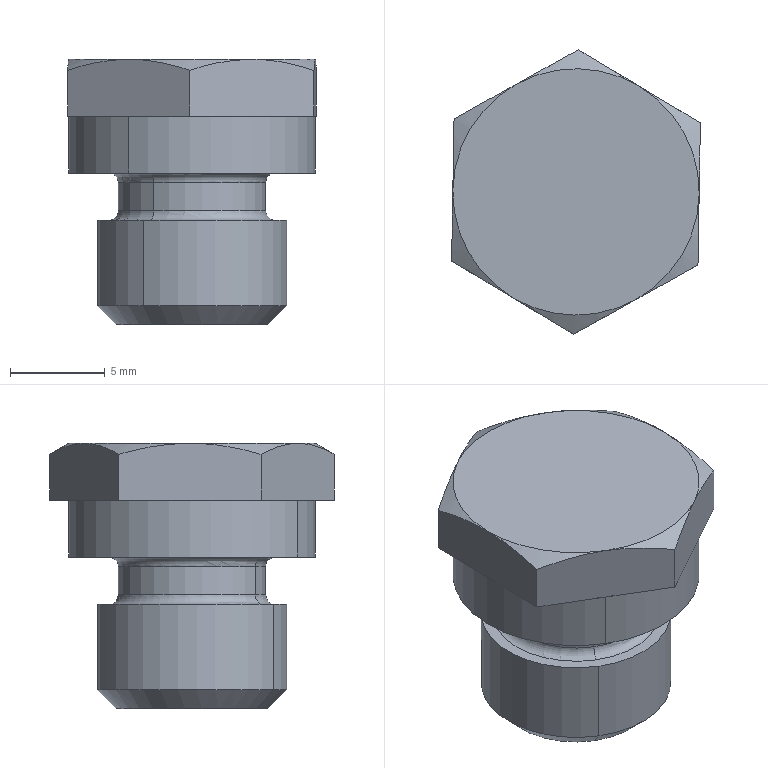Part | SolidWorks | features BaseBody 1 | 1 solid | 34 faces | box 13.126 x 15.009 x 14 mm | volume 1374 mm3 | plane 16 | cone 8 | cylinder 6 | torus 4 | commonest cylinder face diameters 7.8 x2 10 x2 13 x2
STEP:
#1=CARTESIAN_POINT('',(388.093,181.656,45.));
#2=VERTEX_POINT('',#1);
#3=CARTESIAN_POINT('',(392.107,188.344,45.));
#4=VERTEX_POINT('',#3);
#5=CARTESIAN_POINT('',(390.1,185.,45.));
#6=DIRECTION('',(0.,0.,-1.));
#7=DIRECTION('',(0.5146,0.8574,0.));
#8=AXIS2_PLACEMENT_3D('',#5,#6,#7);
#9=CIRCLE('',#8,3.9);
#10=EDGE_CURVE('',#2,#4,#9,.T.);
#11=ORIENTED_EDGE('',*,*,#10,.F.);
#12=CARTESIAN_POINT('',(387.836,181.227,45.5));
#13=VERTEX_POINT('',#12);
#14=CARTESIAN_POINT('',(387.836,181.227,45.));
#15=DIRECTION('',(0.8574,-0.5146,0.));
#16=DIRECTION('',(0.5146,0.8574,0.));
#17=AXIS2_PLACEMENT_3D('',#14,#15,#16);
#18=CIRCLE('',#17,0.5);
#19=EDGE_CURVE('',#2,#13,#18,.T.);
#20=ORIENTED_EDGE('',*,*,#19,.T.);
#21=CARTESIAN_POINT('',(392.364,188.773,45.5));
#22=VERTEX_POINT('',#21);
#23=CARTESIAN_POINT('',(390.1,185.,45.5));
#24=DIRECTION('',(0.,0.,1.));
#25=DIRECTION('',(0.5146,0.8574,0.));
#26=AXIS2_PLACEMENT_3D('',#23,#24,#25);
#27=CIRCLE('',#26,4.4);
#28=EDGE_CURVE('',#22,#13,#27,.T.);
#29=ORIENTED_EDGE('',*,*,#28,.F.);
#30=CARTESIAN_POINT('',(392.364,188.773,45.));
#31=DIRECTION('',(-0.8574,0.5146,0.));
#32=DIRECTION('',(-0.5146,-0.8574,0.));
#33=AXIS2_PLACEMENT_3D('',#30,#31,#32);
#34=CIRCLE('',#33,0.5);
#35=EDGE_CURVE('',#4,#22,#34,.T.);
#36=ORIENTED_EDGE('',*,*,#35,.F.);
#37=EDGE_LOOP('',(#11,#20,#29,#36));
#38=FACE_OUTER_BOUND('',#37,.T.);
#39=CARTESIAN_POINT('',(390.1,185.,45.));
#40=DIRECTION('',(0.,0.,-1.));
#41=DIRECTION('',(0.5146,0.8574,0.));
#42=AXIS2_PLACEMENT_3D('',#39,#40,#41);
#43=TOROIDAL_SURFACE('',#42,4.4,0.5);
#44=ADVANCED_FACE('',(#38),#43,.F.);
#45=CARTESIAN_POINT('',(392.107,188.344,43.5));
#46=VERTEX_POINT('',#45);
#47=CARTESIAN_POINT('',(388.093,181.656,43.5));
#48=VERTEX_POINT('',#47);
#49=CARTESIAN_POINT('',(390.1,185.,43.5));
#50=DIRECTION('',(0.,0.,1.));
#51=DIRECTION('',(-0.5146,-0.8574,0.));
#52=AXIS2_PLACEMENT_3D('',#49,#50,#51);
#53=CIRCLE('',#52,3.9);
#54=EDGE_CURVE('',#46,#48,#53,.T.);
#55=ORIENTED_EDGE('',*,*,#54,.F.);
#56=CARTESIAN_POINT('',(392.364,188.773,43.));
#57=VERTEX_POINT('',#56);
#58=CARTESIAN_POINT('',(392.364,188.773,43.5));
#59=DIRECTION('',(0.8574,-0.5146,0.));
#60=DIRECTION('',(0.5146,0.8574,0.));
#61=AXIS2_PLACEMENT_3D('',#58,#59,#60);
#62=CIRCLE('',#61,0.5);
#63=EDGE_CURVE('',#46,#57,#62,.T.);
#64=ORIENTED_EDGE('',*,*,#63,.T.);
#65=CARTESIAN_POINT('',(387.836,181.227,43.));
#66=VERTEX_POINT('',#65);
#67=CARTESIAN_POINT('',(390.1,185.,43.));
#68=DIRECTION('',(0.,0.,-1.));
#69=DIRECTION('',(-0.5146,-0.8574,0.));
#70=AXIS2_PLACEMENT_3D('',#67,#68,#69);
#71=CIRCLE('',#70,4.4);
#72=EDGE_CURVE('',#66,#57,#71,.T.);
#73=ORIENTED_EDGE('',*,*,#72,.F.);
#74=CARTESIAN_POINT('',(387.836,181.227,43.5));
#75=DIRECTION('',(-0.8574,0.5146,0.));
#76=DIRECTION('',(-0.5146,-0.8574,0.));
#77=AXIS2_PLACEMENT_3D('',#74,#75,#76);
#78=CIRCLE('',#77,0.5);
#79=EDGE_CURVE('',#48,#66,#78,.T.);
#80=ORIENTED_EDGE('',*,*,#79,.F.);
#81=EDGE_LOOP('',(#55,#64,#73,#80));
#82=FACE_OUTER_BOUND('',#81,.T.);
#83=CARTESIAN_POINT('',(390.1,185.,43.5));
#84=DIRECTION('',(0.,0.,1.));
#85=DIRECTION('',(-0.5146,-0.8574,0.));
#86=AXIS2_PLACEMENT_3D('',#83,#84,#85);
#87=TOROIDAL_SURFACE('',#86,4.4,0.5);
#88=ADVANCED_FACE('',(#82),#87,.F.);
#89=CARTESIAN_POINT('',(392.159,188.43,37.5));
#90=VERTEX_POINT('',#89);
#91=CARTESIAN_POINT('',(388.041,181.57,37.5));
#92=VERTEX_POINT('',#91);
#93=CARTESIAN_POINT('',(390.1,185.,37.5));
#94=DIRECTION('',(0.,0.,-1.));
#95=DIRECTION('',(0.5146,0.8574,0.));
#96=AXIS2_PLACEMENT_3D('',#93,#94,#95);
#97=CIRCLE('',#96,4.);
#98=EDGE_CURVE('',#90,#92,#97,.T.);
#99=ORIENTED_EDGE('',*,*,#98,.F.);
#100=CARTESIAN_POINT('',(392.673,189.287,38.5));
#101=VERTEX_POINT('',#100);
#102=CARTESIAN_POINT('',(392.159,188.43,37.5));
#103=DIRECTION('',(0.3639,0.6063,0.7071));
#104=VECTOR('',#103,1000.);
#105=LINE('',#102,#104);
#106=EDGE_CURVE('',#90,#101,#105,.T.);
#107=ORIENTED_EDGE('',*,*,#106,.T.);
#108=CARTESIAN_POINT('',(387.527,180.713,38.5));
#109=VERTEX_POINT('',#108);
#110=CARTESIAN_POINT('',(390.1,185.,38.5));
#111=DIRECTION('',(0.,0.,1.));
#112=DIRECTION('',(0.5146,0.8574,0.));
#113=AXIS2_PLACEMENT_3D('',#110,#111,#112);
#114=CIRCLE('',#113,5.);
#115=EDGE_CURVE('',#109,#101,#114,.T.);
#116=ORIENTED_EDGE('',*,*,#115,.F.);
#117=CARTESIAN_POINT('',(388.041,181.57,37.5));
#118=DIRECTION('',(-0.3639,-0.6063,0.7071));
#119=VECTOR('',#118,1000.);
#120=LINE('',#117,#119);
#121=EDGE_CURVE('',#92,#109,#120,.T.);
#122=ORIENTED_EDGE('',*,*,#121,.F.);
#123=EDGE_LOOP('',(#99,#107,#116,#122));
#124=FACE_OUTER_BOUND('',#123,.T.);
#125=CARTESIAN_POINT('',(390.1,185.,37.5));
#126=DIRECTION('',(0.,0.,1.));
#127=DIRECTION('',(-0.5146,-0.8574,0.));
#128=AXIS2_PLACEMENT_3D('',#125,#126,#127);
#129=CONICAL_SURFACE('',#128,4.,0.7854);
#130=ADVANCED_FACE('',(#124),#129,.T.);
#131=CARTESIAN_POINT('',(392.673,189.287,43.));
#132=VERTEX_POINT('',#131);
#133=CARTESIAN_POINT('',(387.527,180.713,43.));
#134=VERTEX_POINT('',#133);
#135=CARTESIAN_POINT('',(390.1,185.,43.));
#136=DIRECTION('',(0.,0.,-1.));
#137=DIRECTION('',(0.5146,0.8574,0.));
#138=AXIS2_PLACEMENT_3D('',#135,#136,#137);
#139=CIRCLE('',#138,5.);
#140=EDGE_CURVE('',#132,#134,#139,.T.);
#141=ORIENTED_EDGE('',*,*,#140,.T.);
#142=CARTESIAN_POINT('',(387.527,180.713,45.5));
#143=DIRECTION('',(0.,0.,-1.));
#144=VECTOR('',#143,1000.);
#145=LINE('',#142,#144);
#146=EDGE_CURVE('',#134,#109,#145,.T.);
#147=ORIENTED_EDGE('',*,*,#146,.T.);
#148=ORIENTED_EDGE('',*,*,#115,.T.);
#149=CARTESIAN_POINT('',(392.673,189.287,45.5));
#150=DIRECTION('',(0.,0.,-1.));
#151=VECTOR('',#150,1000.);
#152=LINE('',#149,#151);
#153=EDGE_CURVE('',#132,#101,#152,.T.);
#154=ORIENTED_EDGE('',*,*,#153,.F.);
#155=EDGE_LOOP('',(#141,#147,#148,#154));
#156=FACE_OUTER_BOUND('',#155,.T.);
#157=CARTESIAN_POINT('',(390.1,185.,45.5));
#158=DIRECTION('',(0.,0.,-1.));
#159=DIRECTION('',(0.5146,0.8574,0.));
#160=AXIS2_PLACEMENT_3D('',#157,#158,#159);
#161=CYLINDRICAL_SURFACE('',#160,5.);
#162=ADVANCED_FACE('',(#156),#161,.T.);
#163=CARTESIAN_POINT('',(390.1,185.,45.));
#164=DIRECTION('',(0.,0.,-1.));
#165=DIRECTION('',(0.5146,0.8574,0.));
#166=AXIS2_PLACEMENT_3D('',#163,#164,#165);
#167=CIRCLE('',#166,3.9);
#168=EDGE_CURVE('',#4,#2,#167,.T.);
#169=ORIENTED_EDGE('',*,*,#168,.T.);
#170=CARTESIAN_POINT('',(388.093,181.656,36.621));
#171=DIRECTION('',(0.,0.,-1.));
#172=VECTOR('',#171,1000.);
#173=LINE('',#170,#172);
#174=EDGE_CURVE('',#2,#48,#173,.T.);
#175=ORIENTED_EDGE('',*,*,#174,.T.);
#176=CARTESIAN_POINT('',(390.1,185.,43.5));
#177=DIRECTION('',(0.,0.,1.));
#178=DIRECTION('',(-0.5146,-0.8574,0.));
#179=AXIS2_PLACEMENT_3D('',#176,#177,#178);
#180=CIRCLE('',#179,3.9);
#181=EDGE_CURVE('',#48,#46,#180,.T.);
#182=ORIENTED_EDGE('',*,*,#181,.T.);
#183=CARTESIAN_POINT('',(392.107,188.344,36.621));
#184=DIRECTION('',(0.,0.,-1.));
#185=VECTOR('',#184,1000.);
#186=LINE('',#183,#185);
#187=EDGE_CURVE('',#4,#46,#186,.T.);
#188=ORIENTED_EDGE('',*,*,#187,.F.);
#189=EDGE_LOOP('',(#169,#175,#182,#188));
#190=FACE_OUTER_BOUND('',#189,.T.);
#191=CARTESIAN_POINT('',(390.1,185.,36.621));
#192=DIRECTION('',(0.,0.,-1.));
#193=DIRECTION('',(0.5146,0.8574,0.));
#194=AXIS2_PLACEMENT_3D('',#191,#192,#193);
#195=CYLINDRICAL_SURFACE('',#194,3.9);
#196=ADVANCED_FACE('',(#190),#195,.T.);
#197=CARTESIAN_POINT('',(393.254,179.316,48.5));
#198=VERTEX_POINT('',#197);
#199=CARTESIAN_POINT('',(386.755,179.427,48.5));
#200=VERTEX_POINT('',#199);
#201=CARTESIAN_POINT('',(390.1,185.,48.5));
#202=DIRECTION('',(0.,0.,-1.));
#203=DIRECTION('',(0.5146,0.8574,0.));
#204=AXIS2_PLACEMENT_3D('',#201,#202,#203);
#205=CIRCLE('',#204,6.5);
#206=EDGE_CURVE('',#198,#200,#205,.T.);
#207=ORIENTED_EDGE('',*,*,#206,.T.);
#208=CARTESIAN_POINT('',(386.755,179.427,45.5));
#209=VERTEX_POINT('',#208);
#210=CARTESIAN_POINT('',(386.755,179.427,48.5));
#211=DIRECTION('',(0.,0.,-1.));
#212=VECTOR('',#211,1000.);
#213=LINE('',#210,#212);
#214=EDGE_CURVE('',#200,#209,#213,.T.);
#215=ORIENTED_EDGE('',*,*,#214,.T.);
#216=CARTESIAN_POINT('',(393.445,190.573,45.5));
#217=VERTEX_POINT('',#216);
#218=CARTESIAN_POINT('',(390.1,185.,45.5));
#219=DIRECTION('',(0.,0.,1.));
#220=DIRECTION('',(0.5146,0.8574,0.));
#221=AXIS2_PLACEMENT_3D('',#218,#219,#220);
#222=CIRCLE('',#221,6.5);
#223=EDGE_CURVE('',#209,#217,#222,.T.);
#224=ORIENTED_EDGE('',*,*,#223,.T.);
#225=CARTESIAN_POINT('',(393.445,190.573,48.5));
#226=VERTEX_POINT('',#225);
#227=CARTESIAN_POINT('',(393.445,190.573,48.5));
#228=DIRECTION('',(0.,0.,-1.));
#229=VECTOR('',#228,1000.);
#230=LINE('',#227,#229);
#231=EDGE_CURVE('',#226,#217,#230,.T.);
#232=ORIENTED_EDGE('',*,*,#231,.F.);
#233=CARTESIAN_POINT('',(396.599,184.89,48.5));
#234=VERTEX_POINT('',#233);
#235=CARTESIAN_POINT('',(390.1,185.,48.5));
#236=DIRECTION('',(0.,0.,-1.));
#237=DIRECTION('',(0.5146,0.8574,0.));
#238=AXIS2_PLACEMENT_3D('',#235,#236,#237);
#239=CIRCLE('',#238,6.5);
#240=EDGE_CURVE('',#226,#234,#239,.T.);
#241=ORIENTED_EDGE('',*,*,#240,.T.);
#242=CARTESIAN_POINT('',(390.1,185.,48.5));
#243=DIRECTION('',(0.,0.,-1.));
#244=DIRECTION('',(0.5146,0.8574,0.));
#245=AXIS2_PLACEMENT_3D('',#242,#243,#244);
#246=CIRCLE('',#245,6.5);
#247=EDGE_CURVE('',#234,#198,#246,.T.);
#248=ORIENTED_EDGE('',*,*,#247,.T.);
#249=EDGE_LOOP('',(#207,#215,#224,#232,#241,#248));
#250=FACE_OUTER_BOUND('',#249,.T.);
#251=CARTESIAN_POINT('',(390.1,185.,48.5));
#252=DIRECTION('',(0.,0.,-1.));
#253=DIRECTION('',(0.5146,0.8574,0.));
#254=AXIS2_PLACEMENT_3D('',#251,#252,#253);
#255=CYLINDRICAL_SURFACE('',#254,6.5);
#256=ADVANCED_FACE('',(#250),#255,.T.);
#257=CARTESIAN_POINT('',(396.535,181.137,50.919));
#258=VERTEX_POINT('',#257);
#259=CARTESIAN_POINT('',(396.599,184.89,51.5));
#260=VERTEX_POINT('',#259);
#261=CARTESIAN_POINT('',(396.535,181.137,50.919));
#262=CARTESIAN_POINT('',(396.546,181.751,51.097));
#263=CARTESIAN_POINT('',(396.556,182.37,51.243));
#264=CARTESIAN_POINT('',(396.577,183.619,51.445));
#265=CARTESIAN_POINT('',(396.588,184.25,51.5));
#266=CARTESIAN_POINT('',(396.599,184.89,51.5));
#267=B_SPLINE_CURVE_WITH_KNOTS('',3,(#261,#262,#263,#264,#265,#266),.UNSPECIFIED.,.F.,.F.,(4,2,4),(0.000000238,0.001899,0.003797),.UNSPECIFIED.);
#268=EDGE_CURVE('',#258,#260,#267,.T.);
#269=ORIENTED_EDGE('',*,*,#268,.F.);
#270=CARTESIAN_POINT('',(396.535,181.137,48.5));
#271=VERTEX_POINT('',#270);
#272=CARTESIAN_POINT('',(396.535,181.137,37.5));
#273=DIRECTION('',(0.,0.,1.));
#274=VECTOR('',#273,1000.);
#275=LINE('',#272,#274);
#276=EDGE_CURVE('',#271,#258,#275,.T.);
#277=ORIENTED_EDGE('',*,*,#276,.F.);
#278=CARTESIAN_POINT('',(396.663,188.642,48.5));
#279=DIRECTION('',(-0.01698,-0.9999,0.));
#280=VECTOR('',#279,1000.);
#281=LINE('',#278,#280);
#282=EDGE_CURVE('',#234,#271,#281,.T.);
#283=ORIENTED_EDGE('',*,*,#282,.F.);
#284=CARTESIAN_POINT('',(396.663,188.642,48.5));
#285=VERTEX_POINT('',#284);
#286=CARTESIAN_POINT('',(396.663,188.642,48.5));
#287=DIRECTION('',(-0.01698,-0.9999,0.));
#288=VECTOR('',#287,1000.);
#289=LINE('',#286,#288);
#290=EDGE_CURVE('',#285,#234,#289,.T.);
#291=ORIENTED_EDGE('',*,*,#290,.F.);
#292=CARTESIAN_POINT('',(396.663,188.642,50.919));
#293=VERTEX_POINT('',#292);
#294=CARTESIAN_POINT('',(396.663,188.642,37.5));
#295=DIRECTION('',(0.,0.,1.));
#296=VECTOR('',#295,1000.);
#297=LINE('',#294,#296);
#298=EDGE_CURVE('',#285,#293,#297,.T.);
#299=ORIENTED_EDGE('',*,*,#298,.T.);
#300=CARTESIAN_POINT('',(396.599,184.89,51.5));
#301=CARTESIAN_POINT('',(396.604,185.208,51.5));
#302=CARTESIAN_POINT('',(396.61,185.528,51.486));
#303=CARTESIAN_POINT('',(396.621,186.161,51.433));
#304=CARTESIAN_POINT('',(396.626,186.475,51.394));
#305=CARTESIAN_POINT('',(396.642,187.412,51.242));
#306=CARTESIAN_POINT('',(396.652,188.03,51.096));
#307=CARTESIAN_POINT('',(396.663,188.642,50.919));
#308=B_SPLINE_CURVE_WITH_KNOTS('',3,(#300,#301,#302,#303,#304,#305,#306,#307),.UNSPECIFIED.,.F.,.F.,(4,2,2,4),(0.003797,0.004743,0.005689,0.00758),.UNSPECIFIED.);
#309=EDGE_CURVE('',#260,#293,#308,.T.);
#310=ORIENTED_EDGE('',*,*,#309,.F.);
#311=EDGE_LOOP('',(#269,#277,#283,#291,#299,#310));
#312=FACE_OUTER_BOUND('',#311,.T.);
#313=CARTESIAN_POINT('',(396.663,188.642,37.5));
#314=DIRECTION('',(-0.9999,0.01698,0.));
#315=DIRECTION('',(0.01698,0.9999,0.));
#316=AXIS2_PLACEMENT_3D('',#313,#314,#315);
#317=PLANE('',#316);
#318=ADVANCED_FACE('',(#312),#317,.F.);
#319=CARTESIAN_POINT('',(389.973,177.496,50.919));
#320=VERTEX_POINT('',#319);
#321=CARTESIAN_POINT('',(393.254,179.316,51.5));
#322=VERTEX_POINT('',#321);
#323=CARTESIAN_POINT('',(389.973,177.496,50.919));
#324=CARTESIAN_POINT('',(390.509,177.793,51.097));
#325=CARTESIAN_POINT('',(391.05,178.093,51.243));
#326=CARTESIAN_POINT('',(392.143,178.7,51.445));
#327=CARTESIAN_POINT('',(392.695,179.006,51.5));
#328=CARTESIAN_POINT('',(393.254,179.316,51.5));
#329=B_SPLINE_CURVE_WITH_KNOTS('',3,(#323,#324,#325,#326,#327,#328),.UNSPECIFIED.,.F.,.F.,(4,2,4),(0.000000238,0.001899,0.003797),.UNSPECIFIED.);
#330=EDGE_CURVE('',#320,#322,#329,.T.);
#331=ORIENTED_EDGE('',*,*,#330,.F.);
#332=CARTESIAN_POINT('',(389.973,177.496,48.5));
#333=VERTEX_POINT('',#332);
#334=CARTESIAN_POINT('',(389.973,177.496,37.5));
#335=DIRECTION('',(0.,0.,1.));
#336=VECTOR('',#335,1000.);
#337=LINE('',#334,#336);
#338=EDGE_CURVE('',#333,#320,#337,.T.);
#339=ORIENTED_EDGE('',*,*,#338,.F.);
#340=CARTESIAN_POINT('',(396.535,181.137,48.5));
#341=DIRECTION('',(-0.8744,-0.4852,0.));
#342=VECTOR('',#341,1000.);
#343=LINE('',#340,#342);
#344=EDGE_CURVE('',#198,#333,#343,.T.);
#345=ORIENTED_EDGE('',*,*,#344,.F.);
#346=CARTESIAN_POINT('',(396.535,181.137,48.5));
#347=DIRECTION('',(-0.8744,-0.4852,0.));
#348=VECTOR('',#347,1000.);
#349=LINE('',#346,#348);
#350=EDGE_CURVE('',#271,#198,#349,.T.);
#351=ORIENTED_EDGE('',*,*,#350,.F.);
#352=ORIENTED_EDGE('',*,*,#276,.T.);
#353=CARTESIAN_POINT('',(393.254,179.316,51.5));
#354=CARTESIAN_POINT('',(393.532,179.471,51.5));
#355=CARTESIAN_POINT('',(393.812,179.626,51.486));
#356=CARTESIAN_POINT('',(394.366,179.933,51.433));
#357=CARTESIAN_POINT('',(394.64,180.086,51.394));
#358=CARTESIAN_POINT('',(395.46,180.541,51.242));
#359=CARTESIAN_POINT('',(396.,180.84,51.096));
#360=CARTESIAN_POINT('',(396.535,181.137,50.919));
#361=B_SPLINE_CURVE_WITH_KNOTS('',3,(#353,#354,#355,#356,#357,#358,#359,#360),.UNSPECIFIED.,.F.,.F.,(4,2,2,4),(0.003797,0.004743,0.005689,0.00758),.UNSPECIFIED.);
#362=EDGE_CURVE('',#322,#258,#361,.T.);
#363=ORIENTED_EDGE('',*,*,#362,.F.);
#364=EDGE_LOOP('',(#331,#339,#345,#351,#352,#363));
#365=FACE_OUTER_BOUND('',#364,.T.);
#366=CARTESIAN_POINT('',(396.535,181.137,37.5));
#367=DIRECTION('',(-0.4852,0.8744,0.));
#368=DIRECTION('',(0.8744,0.4852,0.));
#369=AXIS2_PLACEMENT_3D('',#366,#367,#368);
#370=PLANE('',#369);
#371=ADVANCED_FACE('',(#365),#370,.F.);
#372=CARTESIAN_POINT('',(383.537,181.358,50.919));
#373=VERTEX_POINT('',#372);
#374=CARTESIAN_POINT('',(386.755,179.427,51.5));
#375=VERTEX_POINT('',#374);
#376=CARTESIAN_POINT('',(383.537,181.358,50.919));
#377=CARTESIAN_POINT('',(384.061,181.043,51.096));
#378=CARTESIAN_POINT('',(384.597,180.722,51.243));
#379=CARTESIAN_POINT('',(385.67,180.078,51.445));
#380=CARTESIAN_POINT('',(386.21,179.754,51.5));
#381=CARTESIAN_POINT('',(386.755,179.427,51.5));
#382=B_SPLINE_CURVE_WITH_KNOTS('',3,(#376,#377,#378,#379,#380,#381),.UNSPECIFIED.,.F.,.F.,(4,2,4),(0.007073,0.008973,0.01087),.UNSPECIFIED.);
#383=EDGE_CURVE('',#373,#375,#382,.T.);
#384=ORIENTED_EDGE('',*,*,#383,.F.);
#385=CARTESIAN_POINT('',(383.537,181.358,48.5));
#386=VERTEX_POINT('',#385);
#387=CARTESIAN_POINT('',(383.537,181.358,37.5));
#388=DIRECTION('',(0.,0.,1.));
#389=VECTOR('',#388,1000.);
#390=LINE('',#387,#389);
#391=EDGE_CURVE('',#386,#373,#390,.T.);
#392=ORIENTED_EDGE('',*,*,#391,.F.);
#393=CARTESIAN_POINT('',(389.973,177.496,48.5));
#394=DIRECTION('',(-0.8574,0.5146,0.));
#395=VECTOR('',#394,1000.);
#396=LINE('',#393,#395);
#397=EDGE_CURVE('',#200,#386,#396,.T.);
#398=ORIENTED_EDGE('',*,*,#397,.F.);
#399=CARTESIAN_POINT('',(389.973,177.496,48.5));
#400=DIRECTION('',(-0.8574,0.5146,0.));
#401=VECTOR('',#400,1000.);
#402=LINE('',#399,#401);
#403=EDGE_CURVE('',#333,#200,#402,.T.);
#404=ORIENTED_EDGE('',*,*,#403,.F.);
#405=ORIENTED_EDGE('',*,*,#338,.T.);
#406=CARTESIAN_POINT('',(386.755,179.427,51.5));
#407=CARTESIAN_POINT('',(387.027,179.263,51.5));
#408=CARTESIAN_POINT('',(387.302,179.098,51.486));
#409=CARTESIAN_POINT('',(387.849,178.77,51.433));
#410=CARTESIAN_POINT('',(388.12,178.607,51.393));
#411=CARTESIAN_POINT('',(388.925,178.124,51.24));
#412=CARTESIAN_POINT('',(389.452,177.808,51.095));
#413=CARTESIAN_POINT('',(389.973,177.496,50.919));
#414=B_SPLINE_CURVE_WITH_KNOTS('',3,(#406,#407,#408,#409,#410,#411,#412,#413),.UNSPECIFIED.,.F.,.F.,(4,2,2,4),(0.01087,0.01182,0.01277,0.01468),.UNSPECIFIED.);
#415=EDGE_CURVE('',#375,#320,#414,.T.);
#416=ORIENTED_EDGE('',*,*,#415,.F.);
#417=EDGE_LOOP('',(#384,#392,#398,#404,#405,#416));
#418=FACE_OUTER_BOUND('',#417,.T.);
#419=CARTESIAN_POINT('',(389.973,177.496,37.5));
#420=DIRECTION('',(0.5146,0.8574,0.));
#421=DIRECTION('',(0.,0.,1.));
#422=AXIS2_PLACEMENT_3D('',#419,#420,#421);
#423=PLANE('',#422);
#424=ADVANCED_FACE('',(#418),#423,.F.);
#425=CARTESIAN_POINT('',(383.665,188.863,50.919));
#426=VERTEX_POINT('',#425);
#427=CARTESIAN_POINT('',(383.601,185.11,51.5));
#428=VERTEX_POINT('',#427);
#429=CARTESIAN_POINT('',(383.665,188.863,50.919));
#430=CARTESIAN_POINT('',(383.654,188.249,51.097));
#431=CARTESIAN_POINT('',(383.644,187.63,51.243));
#432=CARTESIAN_POINT('',(383.623,186.381,51.445));
#433=CARTESIAN_POINT('',(383.612,185.75,51.5));
#434=CARTESIAN_POINT('',(383.601,185.11,51.5));
#435=B_SPLINE_CURVE_WITH_KNOTS('',3,(#429,#430,#431,#432,#433,#434),.UNSPECIFIED.,.F.,.F.,(4,2,4),(0.000000238,0.001899,0.003797),.UNSPECIFIED.);
#436=EDGE_CURVE('',#426,#428,#435,.T.);
#437=ORIENTED_EDGE('',*,*,#436,.F.);
#438=CARTESIAN_POINT('',(383.665,188.863,48.5));
#439=VERTEX_POINT('',#438);
#440=CARTESIAN_POINT('',(383.665,188.863,37.5));
#441=DIRECTION('',(0.,0.,1.));
#442=VECTOR('',#441,1000.);
#443=LINE('',#440,#442);
#444=EDGE_CURVE('',#439,#426,#443,.T.);
#445=ORIENTED_EDGE('',*,*,#444,.F.);
#446=CARTESIAN_POINT('',(383.601,185.11,48.5));
#447=VERTEX_POINT('',#446);
#448=CARTESIAN_POINT('',(383.537,181.358,48.5));
#449=DIRECTION('',(0.01698,0.9999,0.));
#450=VECTOR('',#449,1000.);
#451=LINE('',#448,#450);
#452=EDGE_CURVE('',#447,#439,#451,.T.);
#453=ORIENTED_EDGE('',*,*,#452,.F.);
#454=CARTESIAN_POINT('',(383.537,181.358,48.5));
#455=DIRECTION('',(0.01698,0.9999,0.));
#456=VECTOR('',#455,1000.);
#457=LINE('',#454,#456);
#458=EDGE_CURVE('',#386,#447,#457,.T.);
#459=ORIENTED_EDGE('',*,*,#458,.F.);
#460=ORIENTED_EDGE('',*,*,#391,.T.);
#461=CARTESIAN_POINT('',(383.601,185.11,51.5));
#462=CARTESIAN_POINT('',(383.596,184.792,51.5));
#463=CARTESIAN_POINT('',(383.59,184.472,51.486));
#464=CARTESIAN_POINT('',(383.579,183.839,51.433));
#465=CARTESIAN_POINT('',(383.574,183.525,51.394));
#466=CARTESIAN_POINT('',(383.558,182.588,51.242));
#467=CARTESIAN_POINT('',(383.548,181.97,51.096));
#468=CARTESIAN_POINT('',(383.537,181.358,50.919));
#469=B_SPLINE_CURVE_WITH_KNOTS('',3,(#461,#462,#463,#464,#465,#466,#467,#468),.UNSPECIFIED.,.F.,.F.,(4,2,2,4),(0.003797,0.004743,0.005689,0.00758),.UNSPECIFIED.);
#470=EDGE_CURVE('',#428,#373,#469,.T.);
#471=ORIENTED_EDGE('',*,*,#470,.F.);
#472=EDGE_LOOP('',(#437,#445,#453,#459,#460,#471));
#473=FACE_OUTER_BOUND('',#472,.T.);
#474=CARTESIAN_POINT('',(383.537,181.358,37.5));
#475=DIRECTION('',(0.9999,-0.01698,0.));
#476=DIRECTION('',(-0.01698,-0.9999,0.));
#477=AXIS2_PLACEMENT_3D('',#474,#475,#476);
#478=PLANE('',#477);
#479=ADVANCED_FACE('',(#473),#478,.F.);
#480=CARTESIAN_POINT('',(390.227,192.504,50.919));
#481=VERTEX_POINT('',#480);
#482=CARTESIAN_POINT('',(386.946,190.684,51.5));
#483=VERTEX_POINT('',#482);
#484=CARTESIAN_POINT('',(390.227,192.504,50.919));
#485=CARTESIAN_POINT('',(389.691,192.207,51.097));
#486=CARTESIAN_POINT('',(389.15,191.907,51.243));
#487=CARTESIAN_POINT('',(388.057,191.3,51.445));
#488=CARTESIAN_POINT('',(387.505,190.994,51.5));
#489=CARTESIAN_POINT('',(386.946,190.684,51.5));
#490=B_SPLINE_CURVE_WITH_KNOTS('',3,(#484,#485,#486,#487,#488,#489),.UNSPECIFIED.,.F.,.F.,(4,2,4),(0.000000238,0.001899,0.003797),.UNSPECIFIED.);
#491=EDGE_CURVE('',#481,#483,#490,.T.);
#492=ORIENTED_EDGE('',*,*,#491,.F.);
#493=CARTESIAN_POINT('',(390.227,192.504,48.5));
#494=VERTEX_POINT('',#493);
#495=CARTESIAN_POINT('',(390.227,192.504,37.5));
#496=DIRECTION('',(0.,0.,1.));
#497=VECTOR('',#496,1000.);
#498=LINE('',#495,#497);
#499=EDGE_CURVE('',#494,#481,#498,.T.);
#500=ORIENTED_EDGE('',*,*,#499,.F.);
#501=CARTESIAN_POINT('',(386.946,190.684,48.5));
#502=VERTEX_POINT('',#501);
#503=CARTESIAN_POINT('',(383.665,188.863,48.5));
#504=DIRECTION('',(0.8744,0.4852,0.));
#505=VECTOR('',#504,1000.);
#506=LINE('',#503,#505);
#507=EDGE_CURVE('',#502,#494,#506,.T.);
#508=ORIENTED_EDGE('',*,*,#507,.F.);
#509=CARTESIAN_POINT('',(383.665,188.863,48.5));
#510=DIRECTION('',(0.8744,0.4852,0.));
#511=VECTOR('',#510,1000.);
#512=LINE('',#509,#511);
#513=EDGE_CURVE('',#439,#502,#512,.T.);
#514=ORIENTED_EDGE('',*,*,#513,.F.);
#515=ORIENTED_EDGE('',*,*,#444,.T.);
#516=CARTESIAN_POINT('',(386.946,190.684,51.5));
#517=CARTESIAN_POINT('',(386.668,190.529,51.5));
#518=CARTESIAN_POINT('',(386.388,190.374,51.486));
#519=CARTESIAN_POINT('',(385.834,190.067,51.433));
#520=CARTESIAN_POINT('',(385.56,189.914,51.394));
#521=CARTESIAN_POINT('',(384.74,189.459,51.242));
#522=CARTESIAN_POINT('',(384.2,189.16,51.096));
#523=CARTESIAN_POINT('',(383.665,188.863,50.919));
#524=B_SPLINE_CURVE_WITH_KNOTS('',3,(#516,#517,#518,#519,#520,#521,#522,#523),.UNSPECIFIED.,.F.,.F.,(4,2,2,4),(0.003797,0.004743,0.005689,0.00758),.UNSPECIFIED.);
#525=EDGE_CURVE('',#483,#426,#524,.T.);
#526=ORIENTED_EDGE('',*,*,#525,.F.);
#527=EDGE_LOOP('',(#492,#500,#508,#514,#515,#526));
#528=FACE_OUTER_BOUND('',#527,.T.);
#529=CARTESIAN_POINT('',(383.665,188.863,37.5));
#530=DIRECTION('',(0.4852,-0.8744,0.));
#531=DIRECTION('',(-0.8744,-0.4852,0.));
#532=AXIS2_PLACEMENT_3D('',#529,#530,#531);
#533=PLANE('',#532);
#534=ADVANCED_FACE('',(#528),#533,.F.);
#535=CARTESIAN_POINT('',(393.445,190.573,51.5));
#536=VERTEX_POINT('',#535);
#537=CARTESIAN_POINT('',(396.663,188.642,50.919));
#538=CARTESIAN_POINT('',(396.142,188.954,51.095));
#539=CARTESIAN_POINT('',(395.615,189.271,51.24));
#540=CARTESIAN_POINT('',(394.81,189.754,51.393));
#541=CARTESIAN_POINT('',(394.54,189.916,51.433));
#542=CARTESIAN_POINT('',(393.992,190.245,51.486));
#543=CARTESIAN_POINT('',(393.718,190.41,51.5));
#544=CARTESIAN_POINT('',(393.445,190.573,51.5));
#545=B_SPLINE_CURVE_WITH_KNOTS('',3,(#537,#538,#539,#540,#541,#542,#543,#544),.UNSPECIFIED.,.F.,.F.,(4,2,2,4),(0.01868,0.02058,0.02153,0.02248),.UNSPECIFIED.);
#546=EDGE_CURVE('',#293,#536,#545,.T.);
#547=ORIENTED_EDGE('',*,*,#546,.F.);
#548=ORIENTED_EDGE('',*,*,#298,.F.);
#549=CARTESIAN_POINT('',(390.227,192.504,48.5));
#550=DIRECTION('',(0.8574,-0.5146,0.));
#551=VECTOR('',#550,1000.);
#552=LINE('',#549,#551);
#553=EDGE_CURVE('',#226,#285,#552,.T.);
#554=ORIENTED_EDGE('',*,*,#553,.F.);
#555=CARTESIAN_POINT('',(390.227,192.504,48.5));
#556=DIRECTION('',(0.8574,-0.5146,0.));
#557=VECTOR('',#556,1000.);
#558=LINE('',#555,#557);
#559=EDGE_CURVE('',#494,#226,#558,.T.);
#560=ORIENTED_EDGE('',*,*,#559,.F.);
#561=ORIENTED_EDGE('',*,*,#499,.T.);
#562=CARTESIAN_POINT('',(393.445,190.573,51.5));
#563=CARTESIAN_POINT('',(392.9,190.9,51.5));
#564=CARTESIAN_POINT('',(392.36,191.224,51.445));
#565=CARTESIAN_POINT('',(391.287,191.868,51.243));
#566=CARTESIAN_POINT('',(390.752,192.19,51.096));
#567=CARTESIAN_POINT('',(390.227,192.504,50.919));
#568=B_SPLINE_CURVE_WITH_KNOTS('',3,(#562,#563,#564,#565,#566,#567),.UNSPECIFIED.,.F.,.F.,(4,2,4),(0.02248,0.02438,0.02628),.UNSPECIFIED.);
#569=EDGE_CURVE('',#536,#481,#568,.T.);
#570=ORIENTED_EDGE('',*,*,#569,.F.);
#571=EDGE_LOOP('',(#547,#548,#554,#560,#561,#570));
#572=FACE_OUTER_BOUND('',#571,.T.);
#573=CARTESIAN_POINT('',(390.227,192.504,37.5));
#574=DIRECTION('',(-0.5146,-0.8574,0.));
#575=DIRECTION('',(-0.8574,0.5146,0.));
#576=AXIS2_PLACEMENT_3D('',#573,#574,#575);
#577=PLANE('',#576);
#578=ADVANCED_FACE('',(#572),#577,.F.);
#579=ORIENTED_EDGE('',*,*,#214,.F.);
#580=CARTESIAN_POINT('',(390.1,185.,48.5));
#581=DIRECTION('',(0.,0.,-1.));
#582=DIRECTION('',(0.5146,0.8574,0.));
#583=AXIS2_PLACEMENT_3D('',#580,#581,#582);
#584=CIRCLE('',#583,6.5);
#585=EDGE_CURVE('',#200,#447,#584,.T.);
#586=ORIENTED_EDGE('',*,*,#585,.T.);
#587=CARTESIAN_POINT('',(390.1,185.,48.5));
#588=DIRECTION('',(0.,0.,-1.));
#589=DIRECTION('',(0.5146,0.8574,0.));
#590=AXIS2_PLACEMENT_3D('',#587,#588,#589);
#591=CIRCLE('',#590,6.5);
#592=EDGE_CURVE('',#447,#502,#591,.T.);
#593=ORIENTED_EDGE('',*,*,#592,.T.);
#594=CARTESIAN_POINT('',(390.1,185.,48.5));
#595=DIRECTION('',(0.,0.,-1.));
#596=DIRECTION('',(0.5146,0.8574,0.));
#597=AXIS2_PLACEMENT_3D('',#594,#595,#596);
#598=CIRCLE('',#597,6.5);
#599=EDGE_CURVE('',#502,#226,#598,.T.);
#600=ORIENTED_EDGE('',*,*,#599,.T.);
#601=ORIENTED_EDGE('',*,*,#231,.T.);
#602=CARTESIAN_POINT('',(390.1,185.,45.5));
#603=DIRECTION('',(0.,0.,1.));
#604=DIRECTION('',(0.5146,0.8574,0.));
#605=AXIS2_PLACEMENT_3D('',#602,#603,#604);
#606=CIRCLE('',#605,6.5);
#607=EDGE_CURVE('',#217,#209,#606,.T.);
#608=ORIENTED_EDGE('',*,*,#607,.T.);
#609=EDGE_LOOP('',(#579,#586,#593,#600,#601,#608));
#610=FACE_OUTER_BOUND('',#609,.T.);
#611=CARTESIAN_POINT('',(390.1,185.,48.5));
#612=DIRECTION('',(0.,0.,-1.));
#613=DIRECTION('',(0.5146,0.8574,0.));
#614=AXIS2_PLACEMENT_3D('',#611,#612,#613);
#615=CYLINDRICAL_SURFACE('',#614,6.5);
#616=ADVANCED_FACE('',(#610),#615,.T.);
#617=ORIENTED_EDGE('',*,*,#290,.T.);
#618=ORIENTED_EDGE('',*,*,#240,.F.);
#619=ORIENTED_EDGE('',*,*,#553,.T.);
#620=EDGE_LOOP('',(#617,#618,#619));
#621=FACE_OUTER_BOUND('',#620,.T.);
#622=CARTESIAN_POINT('',(390.1,185.,48.5));
#623=DIRECTION('',(0.,0.,-1.));
#624=DIRECTION('',(0.5146,0.8574,0.));
#625=AXIS2_PLACEMENT_3D('',#622,#623,#624);
#626=PLANE('',#625);
#627=ADVANCED_FACE('',(#621),#626,.T.);
#628=ORIENTED_EDGE('',*,*,#282,.T.);
#629=ORIENTED_EDGE('',*,*,#350,.T.);
#630=ORIENTED_EDGE('',*,*,#247,.F.);
#631=EDGE_LOOP('',(#628,#629,#630));
#632=FACE_OUTER_BOUND('',#631,.T.);
#633=CARTESIAN_POINT('',(390.1,185.,48.5));
#634=DIRECTION('',(0.,0.,-1.));
#635=DIRECTION('',(0.5146,0.8574,0.));
#636=AXIS2_PLACEMENT_3D('',#633,#634,#635);
#637=PLANE('',#636);
#638=ADVANCED_FACE('',(#632),#637,.T.);
#639=ORIENTED_EDGE('',*,*,#344,.T.);
#640=ORIENTED_EDGE('',*,*,#403,.T.);
#641=ORIENTED_EDGE('',*,*,#206,.F.);
#642=EDGE_LOOP('',(#639,#640,#641));
#643=FACE_OUTER_BOUND('',#642,.T.);
#644=CARTESIAN_POINT('',(390.1,185.,48.5));
#645=DIRECTION('',(0.,0.,-1.));
#646=DIRECTION('',(0.5146,0.8574,0.));
#647=AXIS2_PLACEMENT_3D('',#644,#645,#646);
#648=PLANE('',#647);
#649=ADVANCED_FACE('',(#643),#648,.T.);
#650=ORIENTED_EDGE('',*,*,#397,.T.);
#651=ORIENTED_EDGE('',*,*,#458,.T.);
#652=ORIENTED_EDGE('',*,*,#585,.F.);
#653=EDGE_LOOP('',(#650,#651,#652));
#654=FACE_OUTER_BOUND('',#653,.T.);
#655=CARTESIAN_POINT('',(390.1,185.,48.5));
#656=DIRECTION('',(0.,0.,-1.));
#657=DIRECTION('',(0.5146,0.8574,0.));
#658=AXIS2_PLACEMENT_3D('',#655,#656,#657);
#659=PLANE('',#658);
#660=ADVANCED_FACE('',(#654),#659,.T.);
#661=ORIENTED_EDGE('',*,*,#452,.T.);
#662=ORIENTED_EDGE('',*,*,#513,.T.);
#663=ORIENTED_EDGE('',*,*,#592,.F.);
#664=EDGE_LOOP('',(#661,#662,#663));
#665=FACE_OUTER_BOUND('',#664,.T.);
#666=CARTESIAN_POINT('',(390.1,185.,48.5));
#667=DIRECTION('',(0.,0.,-1.));
#668=DIRECTION('',(0.5146,0.8574,0.));
#669=AXIS2_PLACEMENT_3D('',#666,#667,#668);
#670=PLANE('',#669);
#671=ADVANCED_FACE('',(#665),#670,.T.);
#672=ORIENTED_EDGE('',*,*,#507,.T.);
#673=ORIENTED_EDGE('',*,*,#559,.T.);
#674=ORIENTED_EDGE('',*,*,#599,.F.);
#675=EDGE_LOOP('',(#672,#673,#674));
#676=FACE_OUTER_BOUND('',#675,.T.);
#677=CARTESIAN_POINT('',(390.1,185.,48.5));
#678=DIRECTION('',(0.,0.,-1.));
#679=DIRECTION('',(0.5146,0.8574,0.));
#680=AXIS2_PLACEMENT_3D('',#677,#678,#679);
#681=PLANE('',#680);
#682=ADVANCED_FACE('',(#676),#681,.T.);
#683=ORIENTED_EDGE('',*,*,#28,.T.);
#684=CARTESIAN_POINT('',(390.1,185.,45.5));
#685=DIRECTION('',(0.,0.,1.));
#686=DIRECTION('',(0.5146,0.8574,0.));
#687=AXIS2_PLACEMENT_3D('',#684,#685,#686);
#688=CIRCLE('',#687,4.4);
#689=EDGE_CURVE('',#13,#22,#688,.T.);
#690=ORIENTED_EDGE('',*,*,#689,.T.);
#691=EDGE_LOOP('',(#683,#690));
#692=FACE_BOUND('',#691,.T.);
#693=ORIENTED_EDGE('',*,*,#607,.F.);
#694=ORIENTED_EDGE('',*,*,#223,.F.);
#695=EDGE_LOOP('',(#693,#694));
#696=FACE_OUTER_BOUND('',#695,.T.);
#697=CARTESIAN_POINT('',(390.1,185.,45.5));
#698=DIRECTION('',(0.,0.,-1.));
#699=DIRECTION('',(0.5146,0.8574,0.));
#700=AXIS2_PLACEMENT_3D('',#697,#698,#699);
#701=PLANE('',#700);
#702=ADVANCED_FACE('',(#692,#696),#701,.T.);
#703=ORIENTED_EDGE('',*,*,#491,.T.);
#704=CARTESIAN_POINT('',(390.1,185.,51.5));
#705=DIRECTION('',(0.,0.,-1.));
#706=DIRECTION('',(0.5146,0.8574,0.));
#707=AXIS2_PLACEMENT_3D('',#704,#705,#706);
#708=CIRCLE('',#707,6.5);
#709=EDGE_CURVE('',#483,#536,#708,.T.);
#710=ORIENTED_EDGE('',*,*,#709,.T.);
#711=ORIENTED_EDGE('',*,*,#569,.T.);
#712=EDGE_LOOP('',(#703,#710,#711));
#713=FACE_OUTER_BOUND('',#712,.T.);
#714=CARTESIAN_POINT('',(390.1,185.,51.5));
#715=DIRECTION('',(0.,0.,-1.));
#716=DIRECTION('',(-0.5146,-0.8574,0.));
#717=AXIS2_PLACEMENT_3D('',#714,#715,#716);
#718=CONICAL_SURFACE('',#717,6.5,1.047);
#719=ADVANCED_FACE('',(#713),#718,.T.);
#720=ORIENTED_EDGE('',*,*,#436,.T.);
#721=CARTESIAN_POINT('',(390.1,185.,51.5));
#722=DIRECTION('',(0.,0.,-1.));
#723=DIRECTION('',(0.5146,0.8574,0.));
#724=AXIS2_PLACEMENT_3D('',#721,#722,#723);
#725=CIRCLE('',#724,6.5);
#726=EDGE_CURVE('',#428,#483,#725,.T.);
#727=ORIENTED_EDGE('',*,*,#726,.T.);
#728=ORIENTED_EDGE('',*,*,#525,.T.);
#729=EDGE_LOOP('',(#720,#727,#728));
#730=FACE_OUTER_BOUND('',#729,.T.);
#731=CARTESIAN_POINT('',(390.1,185.,51.5));
#732=DIRECTION('',(0.,0.,-1.));
#733=DIRECTION('',(-0.5146,-0.8574,0.));
#734=AXIS2_PLACEMENT_3D('',#731,#732,#733);
#735=CONICAL_SURFACE('',#734,6.5,1.047);
#736=ADVANCED_FACE('',(#730),#735,.T.);
#737=ORIENTED_EDGE('',*,*,#383,.T.);
#738=CARTESIAN_POINT('',(390.1,185.,51.5));
#739=DIRECTION('',(0.,0.,-1.));
#740=DIRECTION('',(0.5146,0.8574,0.));
#741=AXIS2_PLACEMENT_3D('',#738,#739,#740);
#742=CIRCLE('',#741,6.5);
#743=EDGE_CURVE('',#375,#428,#742,.T.);
#744=ORIENTED_EDGE('',*,*,#743,.T.);
#745=ORIENTED_EDGE('',*,*,#470,.T.);
#746=EDGE_LOOP('',(#737,#744,#745));
#747=FACE_OUTER_BOUND('',#746,.T.);
#748=CARTESIAN_POINT('',(390.1,185.,51.5));
#749=DIRECTION('',(0.,0.,-1.));
#750=DIRECTION('',(-0.5146,-0.8574,0.));
#751=AXIS2_PLACEMENT_3D('',#748,#749,#750);
#752=CONICAL_SURFACE('',#751,6.5,1.047);
#753=ADVANCED_FACE('',(#747),#752,.T.);
#754=ORIENTED_EDGE('',*,*,#415,.T.);
#755=ORIENTED_EDGE('',*,*,#330,.T.);
#756=CARTESIAN_POINT('',(390.1,185.,51.5));
#757=DIRECTION('',(0.,0.,1.));
#758=DIRECTION('',(-0.5146,-0.8574,0.));
#759=AXIS2_PLACEMENT_3D('',#756,#757,#758);
#760=CIRCLE('',#759,6.5);
#761=EDGE_CURVE('',#375,#322,#760,.T.);
#762=ORIENTED_EDGE('',*,*,#761,.F.);
#763=EDGE_LOOP('',(#754,#755,#762));
#764=FACE_OUTER_BOUND('',#763,.T.);
#765=CARTESIAN_POINT('',(390.1,185.,51.5));
#766=DIRECTION('',(0.,0.,-1.));
#767=DIRECTION('',(-0.5146,-0.8574,0.));
#768=AXIS2_PLACEMENT_3D('',#765,#766,#767);
#769=CONICAL_SURFACE('',#768,6.5,1.047);
#770=ADVANCED_FACE('',(#764),#769,.T.);
#771=ORIENTED_EDGE('',*,*,#362,.T.);
#772=ORIENTED_EDGE('',*,*,#268,.T.);
#773=CARTESIAN_POINT('',(390.1,185.,51.5));
#774=DIRECTION('',(0.,0.,-1.));
#775=DIRECTION('',(0.5146,0.8574,0.));
#776=AXIS2_PLACEMENT_3D('',#773,#774,#775);
#777=CIRCLE('',#776,6.5);
#778=EDGE_CURVE('',#260,#322,#777,.T.);
#779=ORIENTED_EDGE('',*,*,#778,.T.);
#780=EDGE_LOOP('',(#771,#772,#779));
#781=FACE_OUTER_BOUND('',#780,.T.);
#782=CARTESIAN_POINT('',(390.1,185.,51.5));
#783=DIRECTION('',(0.,0.,-1.));
#784=DIRECTION('',(-0.5146,-0.8574,0.));
#785=AXIS2_PLACEMENT_3D('',#782,#783,#784);
#786=CONICAL_SURFACE('',#785,6.5,1.047);
#787=ADVANCED_FACE('',(#781),#786,.T.);
#788=ORIENTED_EDGE('',*,*,#309,.T.);
#789=ORIENTED_EDGE('',*,*,#546,.T.);
#790=CARTESIAN_POINT('',(390.1,185.,51.5));
#791=DIRECTION('',(0.,0.,-1.));
#792=DIRECTION('',(0.5146,0.8574,0.));
#793=AXIS2_PLACEMENT_3D('',#790,#791,#792);
#794=CIRCLE('',#793,6.5);
#795=EDGE_CURVE('',#536,#260,#794,.T.);
#796=ORIENTED_EDGE('',*,*,#795,.T.);
#797=EDGE_LOOP('',(#788,#789,#796));
#798=FACE_OUTER_BOUND('',#797,.T.);
#799=CARTESIAN_POINT('',(390.1,185.,51.5));
#800=DIRECTION('',(0.,0.,-1.));
#801=DIRECTION('',(-0.5146,-0.8574,0.));
#802=AXIS2_PLACEMENT_3D('',#799,#800,#801);
#803=CONICAL_SURFACE('',#802,6.5,1.047);
#804=ADVANCED_FACE('',(#798),#803,.T.);
#805=ORIENTED_EDGE('',*,*,#795,.F.);
#806=ORIENTED_EDGE('',*,*,#709,.F.);
#807=ORIENTED_EDGE('',*,*,#726,.F.);
#808=ORIENTED_EDGE('',*,*,#743,.F.);
#809=ORIENTED_EDGE('',*,*,#761,.T.);
#810=ORIENTED_EDGE('',*,*,#778,.F.);
#811=EDGE_LOOP('',(#805,#806,#807,#808,#809,#810));
#812=FACE_OUTER_BOUND('',#811,.T.);
#813=CARTESIAN_POINT('',(396.408,173.633,51.5));
#814=DIRECTION('',(0.,0.,-1.));
#815=DIRECTION('',(0.5146,0.8574,0.));
#816=AXIS2_PLACEMENT_3D('',#813,#814,#815);
#817=PLANE('',#816);
#818=ADVANCED_FACE('',(#812),#817,.F.);
#819=ORIENTED_EDGE('',*,*,#72,.T.);
#820=CARTESIAN_POINT('',(390.1,185.,43.));
#821=DIRECTION('',(0.,0.,-1.));
#822=DIRECTION('',(-0.5146,-0.8574,0.));
#823=AXIS2_PLACEMENT_3D('',#820,#821,#822);
#824=CIRCLE('',#823,4.4);
#825=EDGE_CURVE('',#57,#66,#824,.T.);
#826=ORIENTED_EDGE('',*,*,#825,.T.);
#827=EDGE_LOOP('',(#819,#826));
#828=FACE_BOUND('',#827,.T.);
#829=ORIENTED_EDGE('',*,*,#140,.F.);
#830=CARTESIAN_POINT('',(390.1,185.,43.));
#831=DIRECTION('',(0.,0.,-1.));
#832=DIRECTION('',(0.5146,0.8574,0.));
#833=AXIS2_PLACEMENT_3D('',#830,#831,#832);
#834=CIRCLE('',#833,5.);
#835=EDGE_CURVE('',#134,#132,#834,.T.);
#836=ORIENTED_EDGE('',*,*,#835,.F.);
#837=EDGE_LOOP('',(#829,#836));
#838=FACE_OUTER_BOUND('',#837,.T.);
#839=CARTESIAN_POINT('',(394.387,182.427,43.));
#840=DIRECTION('',(0.,0.,1.));
#841=DIRECTION('',(-0.5146,-0.8574,0.));
#842=AXIS2_PLACEMENT_3D('',#839,#840,#841);
#843=PLANE('',#842);
#844=ADVANCED_FACE('',(#828,#838),#843,.T.);
#845=ORIENTED_EDGE('',*,*,#174,.F.);
#846=ORIENTED_EDGE('',*,*,#10,.T.);
#847=ORIENTED_EDGE('',*,*,#187,.T.);
#848=ORIENTED_EDGE('',*,*,#54,.T.);
#849=EDGE_LOOP('',(#845,#846,#847,#848));
#850=FACE_OUTER_BOUND('',#849,.T.);
#851=CARTESIAN_POINT('',(390.1,185.,36.621));
#852=DIRECTION('',(0.,0.,-1.));
#853=DIRECTION('',(0.5146,0.8574,0.));
#854=AXIS2_PLACEMENT_3D('',#851,#852,#853);
#855=CYLINDRICAL_SURFACE('',#854,3.9);
#856=ADVANCED_FACE('',(#850),#855,.T.);
#857=CARTESIAN_POINT('',(390.1,185.,37.5));
#858=DIRECTION('',(0.,0.,-1.));
#859=DIRECTION('',(0.5146,0.8574,0.));
#860=AXIS2_PLACEMENT_3D('',#857,#858,#859);
#861=CIRCLE('',#860,4.);
#862=EDGE_CURVE('',#92,#90,#861,.T.);
#863=ORIENTED_EDGE('',*,*,#862,.T.);
#864=ORIENTED_EDGE('',*,*,#98,.T.);
#865=EDGE_LOOP('',(#863,#864));
#866=FACE_OUTER_BOUND('',#865,.T.);
#867=CARTESIAN_POINT('',(396.408,173.633,37.5));
#868=DIRECTION('',(0.,0.,-1.));
#869=DIRECTION('',(0.5146,0.8574,0.));
#870=AXIS2_PLACEMENT_3D('',#867,#868,#869);
#871=PLANE('',#870);
#872=ADVANCED_FACE('',(#866),#871,.T.);
#873=ORIENTED_EDGE('',*,*,#146,.F.);
#874=ORIENTED_EDGE('',*,*,#835,.T.);
#875=ORIENTED_EDGE('',*,*,#153,.T.);
#876=CARTESIAN_POINT('',(390.1,185.,38.5));
#877=DIRECTION('',(0.,0.,1.));
#878=DIRECTION('',(0.5146,0.8574,0.));
#879=AXIS2_PLACEMENT_3D('',#876,#877,#878);
#880=CIRCLE('',#879,5.);
#881=EDGE_CURVE('',#101,#109,#880,.T.);
#882=ORIENTED_EDGE('',*,*,#881,.T.);
#883=EDGE_LOOP('',(#873,#874,#875,#882));
#884=FACE_OUTER_BOUND('',#883,.T.);
#885=CARTESIAN_POINT('',(390.1,185.,45.5));
#886=DIRECTION('',(0.,0.,-1.));
#887=DIRECTION('',(0.5146,0.8574,0.));
#888=AXIS2_PLACEMENT_3D('',#885,#886,#887);
#889=CYLINDRICAL_SURFACE('',#888,5.);
#890=ADVANCED_FACE('',(#884),#889,.T.);
#891=ORIENTED_EDGE('',*,*,#106,.F.);
#892=ORIENTED_EDGE('',*,*,#862,.F.);
#893=ORIENTED_EDGE('',*,*,#121,.T.);
#894=ORIENTED_EDGE('',*,*,#881,.F.);
#895=EDGE_LOOP('',(#891,#892,#893,#894));
#896=FACE_OUTER_BOUND('',#895,.T.);
#897=CARTESIAN_POINT('',(390.1,185.,37.5));
#898=DIRECTION('',(0.,0.,1.));
#899=DIRECTION('',(-0.5146,-0.8574,0.));
#900=AXIS2_PLACEMENT_3D('',#897,#898,#899);
#901=CONICAL_SURFACE('',#900,4.,0.7854);
#902=ADVANCED_FACE('',(#896),#901,.T.);
#903=ORIENTED_EDGE('',*,*,#63,.F.);
#904=ORIENTED_EDGE('',*,*,#181,.F.);
#905=ORIENTED_EDGE('',*,*,#79,.T.);
#906=ORIENTED_EDGE('',*,*,#825,.F.);
#907=EDGE_LOOP('',(#903,#904,#905,#906));
#908=FACE_OUTER_BOUND('',#907,.T.);
#909=CARTESIAN_POINT('',(390.1,185.,43.5));
#910=DIRECTION('',(0.,0.,1.));
#911=DIRECTION('',(-0.5146,-0.8574,0.));
#912=AXIS2_PLACEMENT_3D('',#909,#910,#911);
#913=TOROIDAL_SURFACE('',#912,4.4,0.5);
#914=ADVANCED_FACE('',(#908),#913,.F.);
#915=ORIENTED_EDGE('',*,*,#19,.F.);
#916=ORIENTED_EDGE('',*,*,#168,.F.);
#917=ORIENTED_EDGE('',*,*,#35,.T.);
#918=ORIENTED_EDGE('',*,*,#689,.F.);
#919=EDGE_LOOP('',(#915,#916,#917,#918));
#920=FACE_OUTER_BOUND('',#919,.T.);
#921=CARTESIAN_POINT('',(390.1,185.,45.));
#922=DIRECTION('',(0.,0.,-1.));
#923=DIRECTION('',(0.5146,0.8574,0.));
#924=AXIS2_PLACEMENT_3D('',#921,#922,#923);
#925=TOROIDAL_SURFACE('',#924,4.4,0.5);
#926=ADVANCED_FACE('',(#920),#925,.F.);
#927=CLOSED_SHELL('',(#44,#88,#130,#162,#196,#256,#318,#371,#424,#479,#534,#578,#616,#627,#638,#649,#660,#671,#682,#702,#719,#736,#753,#770,#787,#804,#818,#844,#856,#872,#890,#902,#914,#926));
#928=MANIFOLD_SOLID_BREP('',#927);
#929=CARTESIAN_POINT('',(0.,0.,0.));
#930=DIRECTION('',(0.,0.,1.));
#931=DIRECTION('',(1.,0.,0.));
#932=AXIS2_PLACEMENT_3D('',#929,#930,#931);
#933=(LENGTH_UNIT()NAMED_UNIT(*)SI_UNIT(.MILLI.,.METRE.));
#934=UNCERTAINTY_MEASURE_WITH_UNIT(LENGTH_MEASURE(0.00001),#933,'','');
#935=(NAMED_UNIT(*)PLANE_ANGLE_UNIT()SI_UNIT($,.RADIAN.));
#936=(NAMED_UNIT(*)SI_UNIT($,.STERADIAN.)SOLID_ANGLE_UNIT());
#937=(GEOMETRIC_REPRESENTATION_CONTEXT(3)GLOBAL_UNCERTAINTY_ASSIGNED_CONTEXT((#934))GLOBAL_UNIT_ASSIGNED_CONTEXT((#933,#935,#936))REPRESENTATION_CONTEXT('',''));
#938=ADVANCED_BREP_SHAPE_REPRESENTATION('',(#928,#932),#937);